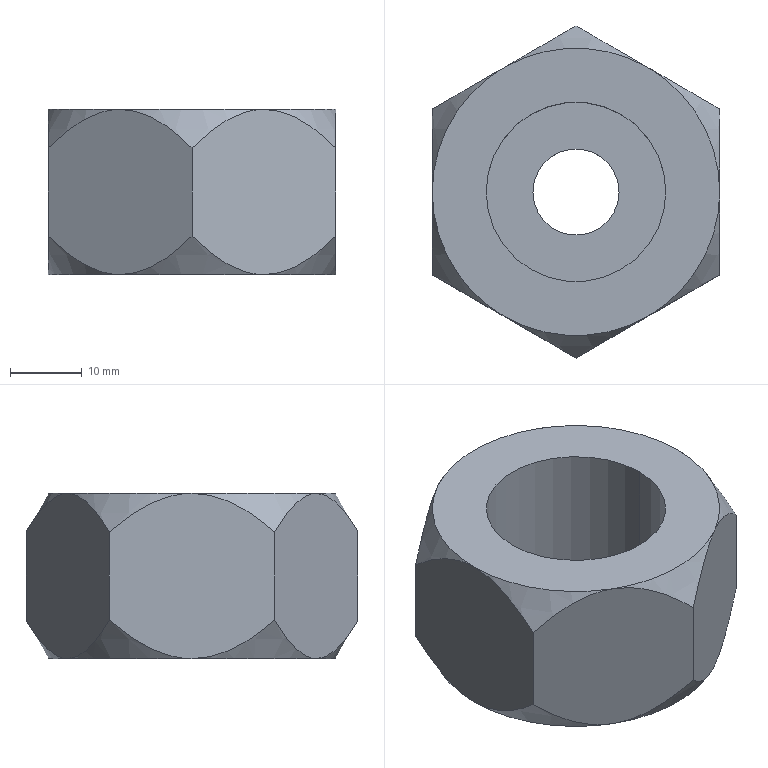Part | SolidWorks | features ICE 3, Extrusion 1, MirrorPattern 1 | 1 solid | 25 faces | box 40 x 46.188 x 23 mm | volume 22052 mm3 | cone 12 | plane 9 | cylinder 4 | commonest cylinder face diameters 12 x2 25 x2
STEP:
#1=CARTESIAN_POINT('',(-6.,0.,-11.5));
#2=VERTEX_POINT('',#1);
#3=CARTESIAN_POINT('',(6.,0.,-11.5));
#4=VERTEX_POINT('',#3);
#5=CARTESIAN_POINT('',(0.,0.,-11.5));
#6=DIRECTION('',(0.,0.,1.));
#7=DIRECTION('',(1.,0.,0.));
#8=AXIS2_PLACEMENT_3D('',#5,#6,#7);
#9=CIRCLE('',#8,6.);
#10=EDGE_CURVE('',#2,#4,#9,.T.);
#11=ORIENTED_EDGE('',*,*,#10,.F.);
#12=CARTESIAN_POINT('',(-6.,0.,-6.5));
#13=VERTEX_POINT('',#12);
#14=CARTESIAN_POINT('',(-6.,0.,-24.5));
#15=DIRECTION('',(0.,0.,1.));
#16=VECTOR('',#15,1000.);
#17=LINE('',#14,#16);
#18=EDGE_CURVE('',#2,#13,#17,.T.);
#19=ORIENTED_EDGE('',*,*,#18,.T.);
#20=CARTESIAN_POINT('',(6.,0.,-6.5));
#21=VERTEX_POINT('',#20);
#22=CARTESIAN_POINT('',(0.,0.,-6.5));
#23=DIRECTION('',(0.,0.,1.));
#24=DIRECTION('',(1.,0.,0.));
#25=AXIS2_PLACEMENT_3D('',#22,#23,#24);
#26=CIRCLE('',#25,6.);
#27=EDGE_CURVE('',#13,#21,#26,.T.);
#28=ORIENTED_EDGE('',*,*,#27,.T.);
#29=CARTESIAN_POINT('',(6.,0.,-24.5));
#30=DIRECTION('',(0.,0.,1.));
#31=VECTOR('',#30,1000.);
#32=LINE('',#29,#31);
#33=EDGE_CURVE('',#4,#21,#32,.T.);
#34=ORIENTED_EDGE('',*,*,#33,.F.);
#35=EDGE_LOOP('',(#11,#19,#28,#34));
#36=FACE_OUTER_BOUND('',#35,.T.);
#37=CARTESIAN_POINT('',(0.,0.,-24.5));
#38=DIRECTION('',(0.,0.,1.));
#39=DIRECTION('',(1.,0.,0.));
#40=AXIS2_PLACEMENT_3D('',#37,#38,#39);
#41=CYLINDRICAL_SURFACE('',#40,6.);
#42=ADVANCED_FACE('',(#36),#41,.F.);
#43=CARTESIAN_POINT('',(-12.5,0.,-6.5));
#44=VERTEX_POINT('',#43);
#45=CARTESIAN_POINT('',(12.5,0.,-6.5));
#46=VERTEX_POINT('',#45);
#47=CARTESIAN_POINT('',(0.,0.,-6.5));
#48=DIRECTION('',(0.,0.,1.));
#49=DIRECTION('',(1.,0.,0.));
#50=AXIS2_PLACEMENT_3D('',#47,#48,#49);
#51=CIRCLE('',#50,12.5);
#52=EDGE_CURVE('',#44,#46,#51,.T.);
#53=ORIENTED_EDGE('',*,*,#52,.F.);
#54=CARTESIAN_POINT('',(-12.5,0.,11.5));
#55=VERTEX_POINT('',#54);
#56=CARTESIAN_POINT('',(-12.5,0.,-6.5));
#57=DIRECTION('',(0.,0.,1.));
#58=VECTOR('',#57,1000.);
#59=LINE('',#56,#58);
#60=EDGE_CURVE('',#44,#55,#59,.T.);
#61=ORIENTED_EDGE('',*,*,#60,.T.);
#62=CARTESIAN_POINT('',(12.5,0.,11.5));
#63=VERTEX_POINT('',#62);
#64=CARTESIAN_POINT('',(0.,0.,11.5));
#65=DIRECTION('',(0.,0.,1.));
#66=DIRECTION('',(1.,0.,0.));
#67=AXIS2_PLACEMENT_3D('',#64,#65,#66);
#68=CIRCLE('',#67,12.5);
#69=EDGE_CURVE('',#55,#63,#68,.T.);
#70=ORIENTED_EDGE('',*,*,#69,.T.);
#71=CARTESIAN_POINT('',(12.5,0.,-6.5));
#72=DIRECTION('',(0.,0.,1.));
#73=VECTOR('',#72,1000.);
#74=LINE('',#71,#73);
#75=EDGE_CURVE('',#46,#63,#74,.T.);
#76=ORIENTED_EDGE('',*,*,#75,.F.);
#77=EDGE_LOOP('',(#53,#61,#70,#76));
#78=FACE_OUTER_BOUND('',#77,.T.);
#79=CARTESIAN_POINT('',(0.,0.,-6.5));
#80=DIRECTION('',(0.,0.,1.));
#81=DIRECTION('',(1.,0.,0.));
#82=AXIS2_PLACEMENT_3D('',#79,#80,#81);
#83=CYLINDRICAL_SURFACE('',#82,12.5);
#84=ADVANCED_FACE('',(#78),#83,.F.);
#85=CARTESIAN_POINT('',(20.,11.547,6.141));
#86=VERTEX_POINT('',#85);
#87=CARTESIAN_POINT('',(20.,11.547,-6.141));
#88=VERTEX_POINT('',#87);
#89=CARTESIAN_POINT('',(20.,11.547,11.5));
#90=DIRECTION('',(0.,0.,-1.));
#91=VECTOR('',#90,1000.);
#92=LINE('',#89,#91);
#93=EDGE_CURVE('',#86,#88,#92,.T.);
#94=ORIENTED_EDGE('',*,*,#93,.T.);
#95=CARTESIAN_POINT('',(10.,17.321,-11.5));
#96=VERTEX_POINT('',#95);
#97=CARTESIAN_POINT('',(20.,11.547,-6.141));
#98=CARTESIAN_POINT('',(19.289,11.958,-6.852));
#99=CARTESIAN_POINT('',(18.557,12.38,-7.528));
#100=CARTESIAN_POINT('',(17.035,13.259,-8.777));
#101=CARTESIAN_POINT('',(16.246,13.715,-9.351));
#102=CARTESIAN_POINT('',(14.996,14.436,-10.097));
#103=CARTESIAN_POINT('',(14.566,14.684,-10.327));
#104=CARTESIAN_POINT('',(13.688,15.191,-10.734));
#105=CARTESIAN_POINT('',(13.243,15.448,-10.909));
#106=CARTESIAN_POINT('',(12.34,15.97,-11.197));
#107=CARTESIAN_POINT('',(11.881,16.235,-11.309));
#108=CARTESIAN_POINT('',(10.947,16.774,-11.461));
#109=CARTESIAN_POINT('',(10.47,17.049,-11.5));
#110=CARTESIAN_POINT('',(10.,17.321,-11.5));
#111=B_SPLINE_CURVE_WITH_KNOTS('',3,(#97,#98,#99,#100,#101,#102,#103,#104,#105,#106,#107,#108,#109,#110),.UNSPECIFIED.,.F.,.F.,(4,2,2,2,2,2,4),(0.000000303,0.003232,0.006463,0.008079,0.009695,0.01131,0.01293),.UNSPECIFIED.);
#112=EDGE_CURVE('',#88,#96,#111,.T.);
#113=ORIENTED_EDGE('',*,*,#112,.T.);
#114=CARTESIAN_POINT('',(0.,23.094,-6.141));
#115=VERTEX_POINT('',#114);
#116=CARTESIAN_POINT('',(10.,17.321,-11.5));
#117=CARTESIAN_POINT('',(9.062,17.862,-11.5));
#118=CARTESIAN_POINT('',(8.137,18.396,-11.347));
#119=CARTESIAN_POINT('',(6.768,19.187,-10.913));
#120=CARTESIAN_POINT('',(6.321,19.444,-10.737));
#121=CARTESIAN_POINT('',(5.452,19.946,-10.336));
#122=CARTESIAN_POINT('',(5.028,20.191,-10.11));
#123=CARTESIAN_POINT('',(4.197,20.671,-9.616));
#124=CARTESIAN_POINT('',(3.791,20.905,-9.349));
#125=CARTESIAN_POINT('',(2.992,21.367,-8.779));
#126=CARTESIAN_POINT('',(2.599,21.594,-8.476));
#127=CARTESIAN_POINT('',(1.447,22.258,-7.532));
#128=CARTESIAN_POINT('',(0.7124,22.683,-6.853));
#129=CARTESIAN_POINT('',(0.,23.094,-6.141));
#130=B_SPLINE_CURVE_WITH_KNOTS('',3,(#116,#117,#118,#119,#120,#121,#122,#123,#124,#125,#126,#127,#128,#129),.UNSPECIFIED.,.F.,.F.,(4,2,2,2,2,2,4),(0.01293,0.01615,0.01777,0.01938,0.02099,0.02261,0.02583),.UNSPECIFIED.);
#131=EDGE_CURVE('',#96,#115,#130,.T.);
#132=ORIENTED_EDGE('',*,*,#131,.T.);
#133=CARTESIAN_POINT('',(0.,23.094,6.141));
#134=VERTEX_POINT('',#133);
#135=CARTESIAN_POINT('',(0.,23.094,11.5));
#136=DIRECTION('',(0.,0.,-1.));
#137=VECTOR('',#136,1000.);
#138=LINE('',#135,#137);
#139=EDGE_CURVE('',#134,#115,#138,.T.);
#140=ORIENTED_EDGE('',*,*,#139,.F.);
#141=CARTESIAN_POINT('',(10.,17.321,11.5));
#142=VERTEX_POINT('',#141);
#143=CARTESIAN_POINT('',(10.,17.321,11.5));
#144=CARTESIAN_POINT('',(9.062,17.862,11.5));
#145=CARTESIAN_POINT('',(8.137,18.396,11.347));
#146=CARTESIAN_POINT('',(6.768,19.187,10.913));
#147=CARTESIAN_POINT('',(6.321,19.444,10.737));
#148=CARTESIAN_POINT('',(5.452,19.946,10.336));
#149=CARTESIAN_POINT('',(5.028,20.191,10.11));
#150=CARTESIAN_POINT('',(4.197,20.671,9.616));
#151=CARTESIAN_POINT('',(3.791,20.905,9.349));
#152=CARTESIAN_POINT('',(2.992,21.367,8.779));
#153=CARTESIAN_POINT('',(2.599,21.594,8.476));
#154=CARTESIAN_POINT('',(1.447,22.258,7.532));
#155=CARTESIAN_POINT('',(0.7124,22.683,6.853));
#156=CARTESIAN_POINT('',(0.,23.094,6.141));
#157=B_SPLINE_CURVE_WITH_KNOTS('',3,(#143,#144,#145,#146,#147,#148,#149,#150,#151,#152,#153,#154,#155,#156),.UNSPECIFIED.,.F.,.F.,(4,2,2,2,2,2,4),(0.01293,0.01615,0.01777,0.01938,0.02099,0.02261,0.02583),.UNSPECIFIED.);
#158=EDGE_CURVE('',#142,#134,#157,.T.);
#159=ORIENTED_EDGE('',*,*,#158,.F.);
#160=CARTESIAN_POINT('',(20.,11.547,6.141));
#161=CARTESIAN_POINT('',(19.289,11.958,6.852));
#162=CARTESIAN_POINT('',(18.557,12.38,7.528));
#163=CARTESIAN_POINT('',(17.035,13.259,8.777));
#164=CARTESIAN_POINT('',(16.246,13.715,9.351));
#165=CARTESIAN_POINT('',(14.996,14.436,10.097));
#166=CARTESIAN_POINT('',(14.566,14.684,10.327));
#167=CARTESIAN_POINT('',(13.688,15.191,10.734));
#168=CARTESIAN_POINT('',(13.243,15.448,10.909));
#169=CARTESIAN_POINT('',(12.34,15.97,11.197));
#170=CARTESIAN_POINT('',(11.881,16.235,11.309));
#171=CARTESIAN_POINT('',(10.947,16.774,11.461));
#172=CARTESIAN_POINT('',(10.47,17.049,11.5));
#173=CARTESIAN_POINT('',(10.,17.321,11.5));
#174=B_SPLINE_CURVE_WITH_KNOTS('',3,(#160,#161,#162,#163,#164,#165,#166,#167,#168,#169,#170,#171,#172,#173),.UNSPECIFIED.,.F.,.F.,(4,2,2,2,2,2,4),(0.000000303,0.003232,0.006463,0.008079,0.009695,0.01131,0.01293),.UNSPECIFIED.);
#175=EDGE_CURVE('',#86,#142,#174,.T.);
#176=ORIENTED_EDGE('',*,*,#175,.F.);
#177=EDGE_LOOP('',(#94,#113,#132,#140,#159,#176));
#178=FACE_OUTER_BOUND('',#177,.T.);
#179=CARTESIAN_POINT('',(20.,11.547,11.5));
#180=DIRECTION('',(-0.5,-0.866,0.));
#181=DIRECTION('',(0.866,-0.5,0.));
#182=AXIS2_PLACEMENT_3D('',#179,#180,#181);
#183=PLANE('',#182);
#184=ADVANCED_FACE('',(#178),#183,.F.);
#185=ORIENTED_EDGE('',*,*,#139,.T.);
#186=CARTESIAN_POINT('',(-10.,17.321,-11.5));
#187=VERTEX_POINT('',#186);
#188=CARTESIAN_POINT('',(0.,23.094,-6.141));
#189=CARTESIAN_POINT('',(-0.7114,22.683,-6.852));
#190=CARTESIAN_POINT('',(-1.443,22.261,-7.528));
#191=CARTESIAN_POINT('',(-2.965,21.382,-8.777));
#192=CARTESIAN_POINT('',(-3.754,20.926,-9.351));
#193=CARTESIAN_POINT('',(-5.004,20.205,-10.097));
#194=CARTESIAN_POINT('',(-5.434,19.957,-10.327));
#195=CARTESIAN_POINT('',(-6.312,19.45,-10.734));
#196=CARTESIAN_POINT('',(-6.757,19.193,-10.909));
#197=CARTESIAN_POINT('',(-7.66,18.671,-11.197));
#198=CARTESIAN_POINT('',(-8.119,18.406,-11.309));
#199=CARTESIAN_POINT('',(-9.053,17.867,-11.461));
#200=CARTESIAN_POINT('',(-9.53,17.592,-11.5));
#201=CARTESIAN_POINT('',(-10.,17.321,-11.5));
#202=B_SPLINE_CURVE_WITH_KNOTS('',3,(#188,#189,#190,#191,#192,#193,#194,#195,#196,#197,#198,#199,#200,#201),.UNSPECIFIED.,.F.,.F.,(4,2,2,2,2,2,4),(0.000000303,0.003232,0.006463,0.008079,0.009695,0.01131,0.01293),.UNSPECIFIED.);
#203=EDGE_CURVE('',#115,#187,#202,.T.);
#204=ORIENTED_EDGE('',*,*,#203,.T.);
#205=CARTESIAN_POINT('',(-20.,11.547,-6.141));
#206=VERTEX_POINT('',#205);
#207=CARTESIAN_POINT('',(-10.,17.321,-11.5));
#208=CARTESIAN_POINT('',(-10.938,16.779,-11.5));
#209=CARTESIAN_POINT('',(-11.863,16.245,-11.347));
#210=CARTESIAN_POINT('',(-13.232,15.454,-10.913));
#211=CARTESIAN_POINT('',(-13.679,15.197,-10.737));
#212=CARTESIAN_POINT('',(-14.548,14.695,-10.336));
#213=CARTESIAN_POINT('',(-14.972,14.45,-10.11));
#214=CARTESIAN_POINT('',(-15.803,13.97,-9.616));
#215=CARTESIAN_POINT('',(-16.209,13.736,-9.349));
#216=CARTESIAN_POINT('',(-17.008,13.274,-8.779));
#217=CARTESIAN_POINT('',(-17.401,13.047,-8.476));
#218=CARTESIAN_POINT('',(-18.553,12.383,-7.532));
#219=CARTESIAN_POINT('',(-19.288,11.958,-6.853));
#220=CARTESIAN_POINT('',(-20.,11.547,-6.141));
#221=B_SPLINE_CURVE_WITH_KNOTS('',3,(#207,#208,#209,#210,#211,#212,#213,#214,#215,#216,#217,#218,#219,#220),.UNSPECIFIED.,.F.,.F.,(4,2,2,2,2,2,4),(0.01293,0.01615,0.01777,0.01938,0.02099,0.02261,0.02583),.UNSPECIFIED.);
#222=EDGE_CURVE('',#187,#206,#221,.T.);
#223=ORIENTED_EDGE('',*,*,#222,.T.);
#224=CARTESIAN_POINT('',(-20.,11.547,6.141));
#225=VERTEX_POINT('',#224);
#226=CARTESIAN_POINT('',(-20.,11.547,11.5));
#227=DIRECTION('',(0.,0.,-1.));
#228=VECTOR('',#227,1000.);
#229=LINE('',#226,#228);
#230=EDGE_CURVE('',#225,#206,#229,.T.);
#231=ORIENTED_EDGE('',*,*,#230,.F.);
#232=CARTESIAN_POINT('',(-10.,17.321,11.5));
#233=VERTEX_POINT('',#232);
#234=CARTESIAN_POINT('',(-10.,17.321,11.5));
#235=CARTESIAN_POINT('',(-10.938,16.779,11.5));
#236=CARTESIAN_POINT('',(-11.863,16.245,11.347));
#237=CARTESIAN_POINT('',(-13.232,15.454,10.913));
#238=CARTESIAN_POINT('',(-13.679,15.197,10.737));
#239=CARTESIAN_POINT('',(-14.548,14.695,10.336));
#240=CARTESIAN_POINT('',(-14.972,14.45,10.11));
#241=CARTESIAN_POINT('',(-15.803,13.97,9.616));
#242=CARTESIAN_POINT('',(-16.209,13.736,9.349));
#243=CARTESIAN_POINT('',(-17.008,13.274,8.779));
#244=CARTESIAN_POINT('',(-17.401,13.047,8.476));
#245=CARTESIAN_POINT('',(-18.553,12.383,7.532));
#246=CARTESIAN_POINT('',(-19.288,11.958,6.853));
#247=CARTESIAN_POINT('',(-20.,11.547,6.141));
#248=B_SPLINE_CURVE_WITH_KNOTS('',3,(#234,#235,#236,#237,#238,#239,#240,#241,#242,#243,#244,#245,#246,#247),.UNSPECIFIED.,.F.,.F.,(4,2,2,2,2,2,4),(0.01293,0.01615,0.01777,0.01938,0.02099,0.02261,0.02583),.UNSPECIFIED.);
#249=EDGE_CURVE('',#233,#225,#248,.T.);
#250=ORIENTED_EDGE('',*,*,#249,.F.);
#251=CARTESIAN_POINT('',(0.,23.094,6.141));
#252=CARTESIAN_POINT('',(-0.7114,22.683,6.852));
#253=CARTESIAN_POINT('',(-1.443,22.261,7.528));
#254=CARTESIAN_POINT('',(-2.965,21.382,8.777));
#255=CARTESIAN_POINT('',(-3.754,20.926,9.351));
#256=CARTESIAN_POINT('',(-5.004,20.205,10.097));
#257=CARTESIAN_POINT('',(-5.434,19.957,10.327));
#258=CARTESIAN_POINT('',(-6.312,19.45,10.734));
#259=CARTESIAN_POINT('',(-6.757,19.193,10.909));
#260=CARTESIAN_POINT('',(-7.66,18.671,11.197));
#261=CARTESIAN_POINT('',(-8.119,18.406,11.309));
#262=CARTESIAN_POINT('',(-9.053,17.867,11.461));
#263=CARTESIAN_POINT('',(-9.53,17.592,11.5));
#264=CARTESIAN_POINT('',(-10.,17.321,11.5));
#265=B_SPLINE_CURVE_WITH_KNOTS('',3,(#251,#252,#253,#254,#255,#256,#257,#258,#259,#260,#261,#262,#263,#264),.UNSPECIFIED.,.F.,.F.,(4,2,2,2,2,2,4),(0.000000303,0.003232,0.006463,0.008079,0.009695,0.01131,0.01293),.UNSPECIFIED.);
#266=EDGE_CURVE('',#134,#233,#265,.T.);
#267=ORIENTED_EDGE('',*,*,#266,.F.);
#268=EDGE_LOOP('',(#185,#204,#223,#231,#250,#267));
#269=FACE_OUTER_BOUND('',#268,.T.);
#270=CARTESIAN_POINT('',(0.,23.094,11.5));
#271=DIRECTION('',(0.5,-0.866,0.));
#272=DIRECTION('',(0.866,0.5,0.));
#273=AXIS2_PLACEMENT_3D('',#270,#271,#272);
#274=PLANE('',#273);
#275=ADVANCED_FACE('',(#269),#274,.F.);
#276=ORIENTED_EDGE('',*,*,#230,.T.);
#277=CARTESIAN_POINT('',(-20.,0.,-11.5));
#278=VERTEX_POINT('',#277);
#279=CARTESIAN_POINT('',(-20.,11.547,-6.141));
#280=CARTESIAN_POINT('',(-20.,11.14,-6.493));
#281=CARTESIAN_POINT('',(-20.,10.726,-6.838));
#282=CARTESIAN_POINT('',(-20.,9.877,-7.511));
#283=CARTESIAN_POINT('',(-20.,9.442,-7.84));
#284=CARTESIAN_POINT('',(-20.,8.115,-8.783));
#285=CARTESIAN_POINT('',(-20.,7.2,-9.358));
#286=CARTESIAN_POINT('',(-20.,5.76,-10.101));
#287=CARTESIAN_POINT('',(-20.,5.269,-10.328));
#288=CARTESIAN_POINT('',(-20.,4.26,-10.733));
#289=CARTESIAN_POINT('',(-20.,3.74,-10.911));
#290=CARTESIAN_POINT('',(-20.,2.693,-11.199));
#291=CARTESIAN_POINT('',(-20.,2.164,-11.31));
#292=CARTESIAN_POINT('',(-20.,1.092,-11.461));
#293=CARTESIAN_POINT('',(-20.,0.5475,-11.5));
#294=CARTESIAN_POINT('',(-20.,0.,-11.5));
#295=B_SPLINE_CURVE_WITH_KNOTS('',3,(#279,#280,#281,#282,#283,#284,#285,#286,#287,#288,#289,#290,#291,#292,#293,#294),.UNSPECIFIED.,.F.,.F.,(4,2,2,2,2,2,2,4),(0.02147,0.02307,0.02467,0.02788,0.02948,0.03108,0.03268,0.03428),.UNSPECIFIED.);
#296=EDGE_CURVE('',#206,#278,#295,.T.);
#297=ORIENTED_EDGE('',*,*,#296,.T.);
#298=CARTESIAN_POINT('',(-20.,-11.547,-6.141));
#299=VERTEX_POINT('',#298);
#300=CARTESIAN_POINT('',(-20.,0.,-11.5));
#301=CARTESIAN_POINT('',(-20.,-1.096,-11.5));
#302=CARTESIAN_POINT('',(-20.,-2.166,-11.344));
#303=CARTESIAN_POINT('',(-20.,-3.74,-10.911));
#304=CARTESIAN_POINT('',(-20.,-4.26,-10.733));
#305=CARTESIAN_POINT('',(-20.,-5.268,-10.328));
#306=CARTESIAN_POINT('',(-20.,-5.759,-10.101));
#307=CARTESIAN_POINT('',(-20.,-7.198,-9.359));
#308=CARTESIAN_POINT('',(-20.,-8.114,-8.784));
#309=CARTESIAN_POINT('',(-20.,-9.443,-7.839));
#310=CARTESIAN_POINT('',(-20.,-9.878,-7.511));
#311=CARTESIAN_POINT('',(-20.,-10.726,-6.838));
#312=CARTESIAN_POINT('',(-20.,-11.14,-6.493));
#313=CARTESIAN_POINT('',(-20.,-11.547,-6.141));
#314=B_SPLINE_CURVE_WITH_KNOTS('',3,(#300,#301,#302,#303,#304,#305,#306,#307,#308,#309,#310,#311,#312,#313),.UNSPECIFIED.,.F.,.F.,(4,2,2,2,2,2,4),(0.03428,0.03749,0.03909,0.04069,0.04389,0.0455,0.0471),.UNSPECIFIED.);
#315=EDGE_CURVE('',#278,#299,#314,.T.);
#316=ORIENTED_EDGE('',*,*,#315,.T.);
#317=CARTESIAN_POINT('',(-20.,-11.547,6.141));
#318=VERTEX_POINT('',#317);
#319=CARTESIAN_POINT('',(-20.,-11.547,11.5));
#320=DIRECTION('',(0.,0.,-1.));
#321=VECTOR('',#320,1000.);
#322=LINE('',#319,#321);
#323=EDGE_CURVE('',#318,#299,#322,.T.);
#324=ORIENTED_EDGE('',*,*,#323,.F.);
#325=CARTESIAN_POINT('',(-20.,0.,11.5));
#326=VERTEX_POINT('',#325);
#327=CARTESIAN_POINT('',(-20.,0.,11.5));
#328=CARTESIAN_POINT('',(-20.,-1.096,11.5));
#329=CARTESIAN_POINT('',(-20.,-2.166,11.344));
#330=CARTESIAN_POINT('',(-20.,-3.74,10.911));
#331=CARTESIAN_POINT('',(-20.,-4.26,10.733));
#332=CARTESIAN_POINT('',(-20.,-5.268,10.328));
#333=CARTESIAN_POINT('',(-20.,-5.759,10.101));
#334=CARTESIAN_POINT('',(-20.,-7.198,9.359));
#335=CARTESIAN_POINT('',(-20.,-8.114,8.784));
#336=CARTESIAN_POINT('',(-20.,-9.443,7.839));
#337=CARTESIAN_POINT('',(-20.,-9.878,7.511));
#338=CARTESIAN_POINT('',(-20.,-10.726,6.838));
#339=CARTESIAN_POINT('',(-20.,-11.14,6.493));
#340=CARTESIAN_POINT('',(-20.,-11.547,6.141));
#341=B_SPLINE_CURVE_WITH_KNOTS('',3,(#327,#328,#329,#330,#331,#332,#333,#334,#335,#336,#337,#338,#339,#340),.UNSPECIFIED.,.F.,.F.,(4,2,2,2,2,2,4),(0.03428,0.03749,0.03909,0.04069,0.04389,0.0455,0.0471),.UNSPECIFIED.);
#342=EDGE_CURVE('',#326,#318,#341,.T.);
#343=ORIENTED_EDGE('',*,*,#342,.F.);
#344=CARTESIAN_POINT('',(-20.,11.547,6.141));
#345=CARTESIAN_POINT('',(-20.,11.14,6.493));
#346=CARTESIAN_POINT('',(-20.,10.726,6.838));
#347=CARTESIAN_POINT('',(-20.,9.877,7.511));
#348=CARTESIAN_POINT('',(-20.,9.442,7.84));
#349=CARTESIAN_POINT('',(-20.,8.115,8.783));
#350=CARTESIAN_POINT('',(-20.,7.2,9.358));
#351=CARTESIAN_POINT('',(-20.,5.76,10.101));
#352=CARTESIAN_POINT('',(-20.,5.269,10.328));
#353=CARTESIAN_POINT('',(-20.,4.26,10.733));
#354=CARTESIAN_POINT('',(-20.,3.74,10.911));
#355=CARTESIAN_POINT('',(-20.,2.693,11.199));
#356=CARTESIAN_POINT('',(-20.,2.164,11.31));
#357=CARTESIAN_POINT('',(-20.,1.092,11.461));
#358=CARTESIAN_POINT('',(-20.,0.5475,11.5));
#359=CARTESIAN_POINT('',(-20.,0.,11.5));
#360=B_SPLINE_CURVE_WITH_KNOTS('',3,(#344,#345,#346,#347,#348,#349,#350,#351,#352,#353,#354,#355,#356,#357,#358,#359),.UNSPECIFIED.,.F.,.F.,(4,2,2,2,2,2,2,4),(0.02147,0.02307,0.02467,0.02788,0.02948,0.03108,0.03268,0.03428),.UNSPECIFIED.);
#361=EDGE_CURVE('',#225,#326,#360,.T.);
#362=ORIENTED_EDGE('',*,*,#361,.F.);
#363=EDGE_LOOP('',(#276,#297,#316,#324,#343,#362));
#364=FACE_OUTER_BOUND('',#363,.T.);
#365=CARTESIAN_POINT('',(-20.,11.547,11.5));
#366=DIRECTION('',(1.,0.,0.));
#367=DIRECTION('',(0.,1.,0.));
#368=AXIS2_PLACEMENT_3D('',#365,#366,#367);
#369=PLANE('',#368);
#370=ADVANCED_FACE('',(#364),#369,.F.);
#371=ORIENTED_EDGE('',*,*,#323,.T.);
#372=CARTESIAN_POINT('',(-10.,-17.321,-11.5));
#373=VERTEX_POINT('',#372);
#374=CARTESIAN_POINT('',(-20.,-11.547,-6.141));
#375=CARTESIAN_POINT('',(-19.289,-11.958,-6.852));
#376=CARTESIAN_POINT('',(-18.557,-12.38,-7.528));
#377=CARTESIAN_POINT('',(-17.035,-13.259,-8.777));
#378=CARTESIAN_POINT('',(-16.246,-13.715,-9.351));
#379=CARTESIAN_POINT('',(-14.996,-14.436,-10.097));
#380=CARTESIAN_POINT('',(-14.566,-14.684,-10.327));
#381=CARTESIAN_POINT('',(-13.688,-15.191,-10.734));
#382=CARTESIAN_POINT('',(-13.243,-15.448,-10.909));
#383=CARTESIAN_POINT('',(-12.34,-15.97,-11.197));
#384=CARTESIAN_POINT('',(-11.881,-16.235,-11.309));
#385=CARTESIAN_POINT('',(-10.947,-16.774,-11.461));
#386=CARTESIAN_POINT('',(-10.47,-17.049,-11.5));
#387=CARTESIAN_POINT('',(-10.,-17.321,-11.5));
#388=B_SPLINE_CURVE_WITH_KNOTS('',3,(#374,#375,#376,#377,#378,#379,#380,#381,#382,#383,#384,#385,#386,#387),.UNSPECIFIED.,.F.,.F.,(4,2,2,2,2,2,4),(0.000000303,0.003232,0.006463,0.008079,0.009695,0.01131,0.01293),.UNSPECIFIED.);
#389=EDGE_CURVE('',#299,#373,#388,.T.);
#390=ORIENTED_EDGE('',*,*,#389,.T.);
#391=CARTESIAN_POINT('',(0.,-23.094,-6.141));
#392=VERTEX_POINT('',#391);
#393=CARTESIAN_POINT('',(-10.,-17.321,-11.5));
#394=CARTESIAN_POINT('',(-9.062,-17.862,-11.5));
#395=CARTESIAN_POINT('',(-8.137,-18.396,-11.347));
#396=CARTESIAN_POINT('',(-6.768,-19.187,-10.913));
#397=CARTESIAN_POINT('',(-6.321,-19.444,-10.737));
#398=CARTESIAN_POINT('',(-5.452,-19.946,-10.336));
#399=CARTESIAN_POINT('',(-5.028,-20.191,-10.11));
#400=CARTESIAN_POINT('',(-4.197,-20.671,-9.616));
#401=CARTESIAN_POINT('',(-3.791,-20.905,-9.349));
#402=CARTESIAN_POINT('',(-2.992,-21.367,-8.779));
#403=CARTESIAN_POINT('',(-2.599,-21.594,-8.476));
#404=CARTESIAN_POINT('',(-1.447,-22.258,-7.532));
#405=CARTESIAN_POINT('',(-0.7124,-22.683,-6.853));
#406=CARTESIAN_POINT('',(0.,-23.094,-6.141));
#407=B_SPLINE_CURVE_WITH_KNOTS('',3,(#393,#394,#395,#396,#397,#398,#399,#400,#401,#402,#403,#404,#405,#406),.UNSPECIFIED.,.F.,.F.,(4,2,2,2,2,2,4),(0.01293,0.01615,0.01777,0.01938,0.02099,0.02261,0.02583),.UNSPECIFIED.);
#408=EDGE_CURVE('',#373,#392,#407,.T.);
#409=ORIENTED_EDGE('',*,*,#408,.T.);
#410=CARTESIAN_POINT('',(0.,-23.094,6.141));
#411=VERTEX_POINT('',#410);
#412=CARTESIAN_POINT('',(0.,-23.094,11.5));
#413=DIRECTION('',(0.,0.,-1.));
#414=VECTOR('',#413,1000.);
#415=LINE('',#412,#414);
#416=EDGE_CURVE('',#411,#392,#415,.T.);
#417=ORIENTED_EDGE('',*,*,#416,.F.);
#418=CARTESIAN_POINT('',(-10.,-17.321,11.5));
#419=VERTEX_POINT('',#418);
#420=CARTESIAN_POINT('',(-10.,-17.321,11.5));
#421=CARTESIAN_POINT('',(-9.062,-17.862,11.5));
#422=CARTESIAN_POINT('',(-8.137,-18.396,11.347));
#423=CARTESIAN_POINT('',(-6.768,-19.187,10.913));
#424=CARTESIAN_POINT('',(-6.321,-19.444,10.737));
#425=CARTESIAN_POINT('',(-5.452,-19.946,10.336));
#426=CARTESIAN_POINT('',(-5.028,-20.191,10.11));
#427=CARTESIAN_POINT('',(-4.197,-20.671,9.616));
#428=CARTESIAN_POINT('',(-3.791,-20.905,9.349));
#429=CARTESIAN_POINT('',(-2.992,-21.367,8.779));
#430=CARTESIAN_POINT('',(-2.599,-21.594,8.476));
#431=CARTESIAN_POINT('',(-1.447,-22.258,7.532));
#432=CARTESIAN_POINT('',(-0.7124,-22.683,6.853));
#433=CARTESIAN_POINT('',(0.,-23.094,6.141));
#434=B_SPLINE_CURVE_WITH_KNOTS('',3,(#420,#421,#422,#423,#424,#425,#426,#427,#428,#429,#430,#431,#432,#433),.UNSPECIFIED.,.F.,.F.,(4,2,2,2,2,2,4),(0.01293,0.01615,0.01777,0.01938,0.02099,0.02261,0.02583),.UNSPECIFIED.);
#435=EDGE_CURVE('',#419,#411,#434,.T.);
#436=ORIENTED_EDGE('',*,*,#435,.F.);
#437=CARTESIAN_POINT('',(-20.,-11.547,6.141));
#438=CARTESIAN_POINT('',(-19.289,-11.958,6.852));
#439=CARTESIAN_POINT('',(-18.557,-12.38,7.528));
#440=CARTESIAN_POINT('',(-17.035,-13.259,8.777));
#441=CARTESIAN_POINT('',(-16.246,-13.715,9.351));
#442=CARTESIAN_POINT('',(-14.996,-14.436,10.097));
#443=CARTESIAN_POINT('',(-14.566,-14.684,10.327));
#444=CARTESIAN_POINT('',(-13.688,-15.191,10.734));
#445=CARTESIAN_POINT('',(-13.243,-15.448,10.909));
#446=CARTESIAN_POINT('',(-12.34,-15.97,11.197));
#447=CARTESIAN_POINT('',(-11.881,-16.235,11.309));
#448=CARTESIAN_POINT('',(-10.947,-16.774,11.461));
#449=CARTESIAN_POINT('',(-10.47,-17.049,11.5));
#450=CARTESIAN_POINT('',(-10.,-17.321,11.5));
#451=B_SPLINE_CURVE_WITH_KNOTS('',3,(#437,#438,#439,#440,#441,#442,#443,#444,#445,#446,#447,#448,#449,#450),.UNSPECIFIED.,.F.,.F.,(4,2,2,2,2,2,4),(0.000000303,0.003232,0.006463,0.008079,0.009695,0.01131,0.01293),.UNSPECIFIED.);
#452=EDGE_CURVE('',#318,#419,#451,.T.);
#453=ORIENTED_EDGE('',*,*,#452,.F.);
#454=EDGE_LOOP('',(#371,#390,#409,#417,#436,#453));
#455=FACE_OUTER_BOUND('',#454,.T.);
#456=CARTESIAN_POINT('',(-20.,-11.547,11.5));
#457=DIRECTION('',(0.5,0.866,0.));
#458=DIRECTION('',(-0.866,0.5,0.));
#459=AXIS2_PLACEMENT_3D('',#456,#457,#458);
#460=PLANE('',#459);
#461=ADVANCED_FACE('',(#455),#460,.F.);
#462=ORIENTED_EDGE('',*,*,#416,.T.);
#463=CARTESIAN_POINT('',(10.,-17.321,-11.5));
#464=VERTEX_POINT('',#463);
#465=CARTESIAN_POINT('',(0.,-23.094,-6.141));
#466=CARTESIAN_POINT('',(0.7114,-22.683,-6.852));
#467=CARTESIAN_POINT('',(1.443,-22.261,-7.528));
#468=CARTESIAN_POINT('',(2.965,-21.382,-8.777));
#469=CARTESIAN_POINT('',(3.754,-20.926,-9.351));
#470=CARTESIAN_POINT('',(5.004,-20.205,-10.097));
#471=CARTESIAN_POINT('',(5.434,-19.957,-10.327));
#472=CARTESIAN_POINT('',(6.312,-19.45,-10.734));
#473=CARTESIAN_POINT('',(6.757,-19.193,-10.909));
#474=CARTESIAN_POINT('',(7.66,-18.671,-11.197));
#475=CARTESIAN_POINT('',(8.119,-18.406,-11.309));
#476=CARTESIAN_POINT('',(9.053,-17.867,-11.461));
#477=CARTESIAN_POINT('',(9.53,-17.592,-11.5));
#478=CARTESIAN_POINT('',(10.,-17.321,-11.5));
#479=B_SPLINE_CURVE_WITH_KNOTS('',3,(#465,#466,#467,#468,#469,#470,#471,#472,#473,#474,#475,#476,#477,#478),.UNSPECIFIED.,.F.,.F.,(4,2,2,2,2,2,4),(0.000000303,0.003232,0.006463,0.008079,0.009695,0.01131,0.01293),.UNSPECIFIED.);
#480=EDGE_CURVE('',#392,#464,#479,.T.);
#481=ORIENTED_EDGE('',*,*,#480,.T.);
#482=CARTESIAN_POINT('',(20.,-11.547,-6.141));
#483=VERTEX_POINT('',#482);
#484=CARTESIAN_POINT('',(10.,-17.321,-11.5));
#485=CARTESIAN_POINT('',(10.938,-16.779,-11.5));
#486=CARTESIAN_POINT('',(11.863,-16.245,-11.347));
#487=CARTESIAN_POINT('',(13.232,-15.454,-10.913));
#488=CARTESIAN_POINT('',(13.679,-15.197,-10.737));
#489=CARTESIAN_POINT('',(14.548,-14.695,-10.336));
#490=CARTESIAN_POINT('',(14.972,-14.45,-10.11));
#491=CARTESIAN_POINT('',(15.803,-13.97,-9.616));
#492=CARTESIAN_POINT('',(16.209,-13.736,-9.349));
#493=CARTESIAN_POINT('',(17.008,-13.274,-8.779));
#494=CARTESIAN_POINT('',(17.401,-13.047,-8.476));
#495=CARTESIAN_POINT('',(18.553,-12.383,-7.532));
#496=CARTESIAN_POINT('',(19.288,-11.958,-6.853));
#497=CARTESIAN_POINT('',(20.,-11.547,-6.141));
#498=B_SPLINE_CURVE_WITH_KNOTS('',3,(#484,#485,#486,#487,#488,#489,#490,#491,#492,#493,#494,#495,#496,#497),.UNSPECIFIED.,.F.,.F.,(4,2,2,2,2,2,4),(0.01293,0.01615,0.01777,0.01938,0.02099,0.02261,0.02583),.UNSPECIFIED.);
#499=EDGE_CURVE('',#464,#483,#498,.T.);
#500=ORIENTED_EDGE('',*,*,#499,.T.);
#501=CARTESIAN_POINT('',(20.,-11.547,6.141));
#502=VERTEX_POINT('',#501);
#503=CARTESIAN_POINT('',(20.,-11.547,11.5));
#504=DIRECTION('',(0.,0.,-1.));
#505=VECTOR('',#504,1000.);
#506=LINE('',#503,#505);
#507=EDGE_CURVE('',#502,#483,#506,.T.);
#508=ORIENTED_EDGE('',*,*,#507,.F.);
#509=CARTESIAN_POINT('',(10.,-17.321,11.5));
#510=VERTEX_POINT('',#509);
#511=CARTESIAN_POINT('',(10.,-17.321,11.5));
#512=CARTESIAN_POINT('',(10.938,-16.779,11.5));
#513=CARTESIAN_POINT('',(11.863,-16.245,11.347));
#514=CARTESIAN_POINT('',(13.232,-15.454,10.913));
#515=CARTESIAN_POINT('',(13.679,-15.197,10.737));
#516=CARTESIAN_POINT('',(14.548,-14.695,10.336));
#517=CARTESIAN_POINT('',(14.972,-14.45,10.11));
#518=CARTESIAN_POINT('',(15.803,-13.97,9.616));
#519=CARTESIAN_POINT('',(16.209,-13.736,9.349));
#520=CARTESIAN_POINT('',(17.008,-13.274,8.779));
#521=CARTESIAN_POINT('',(17.401,-13.047,8.476));
#522=CARTESIAN_POINT('',(18.553,-12.383,7.532));
#523=CARTESIAN_POINT('',(19.288,-11.958,6.853));
#524=CARTESIAN_POINT('',(20.,-11.547,6.141));
#525=B_SPLINE_CURVE_WITH_KNOTS('',3,(#511,#512,#513,#514,#515,#516,#517,#518,#519,#520,#521,#522,#523,#524),.UNSPECIFIED.,.F.,.F.,(4,2,2,2,2,2,4),(0.01293,0.01615,0.01777,0.01938,0.02099,0.02261,0.02583),.UNSPECIFIED.);
#526=EDGE_CURVE('',#510,#502,#525,.T.);
#527=ORIENTED_EDGE('',*,*,#526,.F.);
#528=CARTESIAN_POINT('',(0.,-23.094,6.141));
#529=CARTESIAN_POINT('',(0.7114,-22.683,6.852));
#530=CARTESIAN_POINT('',(1.443,-22.261,7.528));
#531=CARTESIAN_POINT('',(2.965,-21.382,8.777));
#532=CARTESIAN_POINT('',(3.754,-20.926,9.351));
#533=CARTESIAN_POINT('',(5.004,-20.205,10.097));
#534=CARTESIAN_POINT('',(5.434,-19.957,10.327));
#535=CARTESIAN_POINT('',(6.312,-19.45,10.734));
#536=CARTESIAN_POINT('',(6.757,-19.193,10.909));
#537=CARTESIAN_POINT('',(7.66,-18.671,11.197));
#538=CARTESIAN_POINT('',(8.119,-18.406,11.309));
#539=CARTESIAN_POINT('',(9.053,-17.867,11.461));
#540=CARTESIAN_POINT('',(9.53,-17.592,11.5));
#541=CARTESIAN_POINT('',(10.,-17.321,11.5));
#542=B_SPLINE_CURVE_WITH_KNOTS('',3,(#528,#529,#530,#531,#532,#533,#534,#535,#536,#537,#538,#539,#540,#541),.UNSPECIFIED.,.F.,.F.,(4,2,2,2,2,2,4),(0.000000303,0.003232,0.006463,0.008079,0.009695,0.01131,0.01293),.UNSPECIFIED.);
#543=EDGE_CURVE('',#411,#510,#542,.T.);
#544=ORIENTED_EDGE('',*,*,#543,.F.);
#545=EDGE_LOOP('',(#462,#481,#500,#508,#527,#544));
#546=FACE_OUTER_BOUND('',#545,.T.);
#547=CARTESIAN_POINT('',(0.,-23.094,11.5));
#548=DIRECTION('',(-0.5,0.866,0.));
#549=DIRECTION('',(-0.866,-0.5,0.));
#550=AXIS2_PLACEMENT_3D('',#547,#548,#549);
#551=PLANE('',#550);
#552=ADVANCED_FACE('',(#546),#551,.F.);
#553=ORIENTED_EDGE('',*,*,#507,.T.);
#554=CARTESIAN_POINT('',(20.,0.,-11.5));
#555=VERTEX_POINT('',#554);
#556=CARTESIAN_POINT('',(20.,-11.547,-6.141));
#557=CARTESIAN_POINT('',(20.,-11.14,-6.493));
#558=CARTESIAN_POINT('',(20.,-10.726,-6.838));
#559=CARTESIAN_POINT('',(20.,-9.878,-7.511));
#560=CARTESIAN_POINT('',(20.,-9.443,-7.839));
#561=CARTESIAN_POINT('',(20.,-8.114,-8.784));
#562=CARTESIAN_POINT('',(20.,-7.198,-9.359));
#563=CARTESIAN_POINT('',(20.,-5.759,-10.101));
#564=CARTESIAN_POINT('',(20.,-5.268,-10.328));
#565=CARTESIAN_POINT('',(20.,-4.26,-10.733));
#566=CARTESIAN_POINT('',(20.,-3.74,-10.911));
#567=CARTESIAN_POINT('',(20.,-2.166,-11.344));
#568=CARTESIAN_POINT('',(20.,-1.096,-11.5));
#569=CARTESIAN_POINT('',(20.,0.,-11.5));
#570=B_SPLINE_CURVE_WITH_KNOTS('',3,(#556,#557,#558,#559,#560,#561,#562,#563,#564,#565,#566,#567,#568,#569),.UNSPECIFIED.,.F.,.F.,(4,2,2,2,2,2,4),(0.01673,0.01834,0.01995,0.02316,0.02476,0.02637,0.02958),.UNSPECIFIED.);
#571=EDGE_CURVE('',#483,#555,#570,.T.);
#572=ORIENTED_EDGE('',*,*,#571,.T.);
#573=CARTESIAN_POINT('',(20.,0.,-11.5));
#574=CARTESIAN_POINT('',(20.,0.5475,-11.5));
#575=CARTESIAN_POINT('',(20.,1.092,-11.461));
#576=CARTESIAN_POINT('',(20.,2.164,-11.31));
#577=CARTESIAN_POINT('',(20.,2.693,-11.199));
#578=CARTESIAN_POINT('',(20.,3.74,-10.911));
#579=CARTESIAN_POINT('',(20.,4.26,-10.733));
#580=CARTESIAN_POINT('',(20.,5.269,-10.328));
#581=CARTESIAN_POINT('',(20.,5.76,-10.101));
#582=CARTESIAN_POINT('',(20.,7.2,-9.358));
#583=CARTESIAN_POINT('',(20.,8.115,-8.783));
#584=CARTESIAN_POINT('',(20.,9.442,-7.84));
#585=CARTESIAN_POINT('',(20.,9.877,-7.511));
#586=CARTESIAN_POINT('',(20.,10.726,-6.838));
#587=CARTESIAN_POINT('',(20.,11.14,-6.493));
#588=CARTESIAN_POINT('',(20.,11.547,-6.141));
#589=B_SPLINE_CURVE_WITH_KNOTS('',3,(#573,#574,#575,#576,#577,#578,#579,#580,#581,#582,#583,#584,#585,#586,#587,#588),.UNSPECIFIED.,.F.,.F.,(4,2,2,2,2,2,2,4),(0.02958,0.03119,0.03279,0.0344,0.03601,0.03922,0.04082,0.04243),.UNSPECIFIED.);
#590=EDGE_CURVE('',#555,#88,#589,.T.);
#591=ORIENTED_EDGE('',*,*,#590,.T.);
#592=ORIENTED_EDGE('',*,*,#93,.F.);
#593=CARTESIAN_POINT('',(20.,0.,11.5));
#594=VERTEX_POINT('',#593);
#595=CARTESIAN_POINT('',(20.,0.,11.5));
#596=CARTESIAN_POINT('',(20.,0.5475,11.5));
#597=CARTESIAN_POINT('',(20.,1.092,11.461));
#598=CARTESIAN_POINT('',(20.,2.164,11.31));
#599=CARTESIAN_POINT('',(20.,2.693,11.199));
#600=CARTESIAN_POINT('',(20.,3.74,10.911));
#601=CARTESIAN_POINT('',(20.,4.26,10.733));
#602=CARTESIAN_POINT('',(20.,5.269,10.328));
#603=CARTESIAN_POINT('',(20.,5.76,10.101));
#604=CARTESIAN_POINT('',(20.,7.2,9.358));
#605=CARTESIAN_POINT('',(20.,8.115,8.783));
#606=CARTESIAN_POINT('',(20.,9.442,7.84));
#607=CARTESIAN_POINT('',(20.,9.877,7.511));
#608=CARTESIAN_POINT('',(20.,10.726,6.838));
#609=CARTESIAN_POINT('',(20.,11.14,6.493));
#610=CARTESIAN_POINT('',(20.,11.547,6.141));
#611=B_SPLINE_CURVE_WITH_KNOTS('',3,(#595,#596,#597,#598,#599,#600,#601,#602,#603,#604,#605,#606,#607,#608,#609,#610),.UNSPECIFIED.,.F.,.F.,(4,2,2,2,2,2,2,4),(0.02958,0.03119,0.03279,0.0344,0.03601,0.03922,0.04082,0.04243),.UNSPECIFIED.);
#612=EDGE_CURVE('',#594,#86,#611,.T.);
#613=ORIENTED_EDGE('',*,*,#612,.F.);
#614=CARTESIAN_POINT('',(20.,-11.547,6.141));
#615=CARTESIAN_POINT('',(20.,-11.14,6.493));
#616=CARTESIAN_POINT('',(20.,-10.726,6.838));
#617=CARTESIAN_POINT('',(20.,-9.878,7.511));
#618=CARTESIAN_POINT('',(20.,-9.443,7.839));
#619=CARTESIAN_POINT('',(20.,-8.114,8.784));
#620=CARTESIAN_POINT('',(20.,-7.198,9.359));
#621=CARTESIAN_POINT('',(20.,-5.759,10.101));
#622=CARTESIAN_POINT('',(20.,-5.268,10.328));
#623=CARTESIAN_POINT('',(20.,-4.26,10.733));
#624=CARTESIAN_POINT('',(20.,-3.74,10.911));
#625=CARTESIAN_POINT('',(20.,-2.166,11.344));
#626=CARTESIAN_POINT('',(20.,-1.096,11.5));
#627=CARTESIAN_POINT('',(20.,0.,11.5));
#628=B_SPLINE_CURVE_WITH_KNOTS('',3,(#614,#615,#616,#617,#618,#619,#620,#621,#622,#623,#624,#625,#626,#627),.UNSPECIFIED.,.F.,.F.,(4,2,2,2,2,2,4),(0.01673,0.01834,0.01995,0.02316,0.02476,0.02637,0.02958),.UNSPECIFIED.);
#629=EDGE_CURVE('',#502,#594,#628,.T.);
#630=ORIENTED_EDGE('',*,*,#629,.F.);
#631=EDGE_LOOP('',(#553,#572,#591,#592,#613,#630));
#632=FACE_OUTER_BOUND('',#631,.T.);
#633=CARTESIAN_POINT('',(20.,-11.547,11.5));
#634=DIRECTION('',(-1.,0.,0.));
#635=DIRECTION('',(0.,-1.,0.));
#636=AXIS2_PLACEMENT_3D('',#633,#634,#635);
#637=PLANE('',#636);
#638=ADVANCED_FACE('',(#632),#637,.F.);
#639=ORIENTED_EDGE('',*,*,#526,.T.);
#640=ORIENTED_EDGE('',*,*,#629,.T.);
#641=CARTESIAN_POINT('',(0.,0.,11.5));
#642=DIRECTION('',(0.,0.,1.));
#643=DIRECTION('',(1.,0.,0.));
#644=AXIS2_PLACEMENT_3D('',#641,#642,#643);
#645=CIRCLE('',#644,20.);
#646=EDGE_CURVE('',#510,#594,#645,.T.);
#647=ORIENTED_EDGE('',*,*,#646,.F.);
#648=EDGE_LOOP('',(#639,#640,#647));
#649=FACE_OUTER_BOUND('',#648,.T.);
#650=CARTESIAN_POINT('',(0.,0.,11.5));
#651=DIRECTION('',(0.,0.,-1.));
#652=DIRECTION('',(1.,0.,0.));
#653=AXIS2_PLACEMENT_3D('',#650,#651,#652);
#654=CONICAL_SURFACE('',#653,20.,0.5236);
#655=ADVANCED_FACE('',(#649),#654,.T.);
#656=ORIENTED_EDGE('',*,*,#435,.T.);
#657=ORIENTED_EDGE('',*,*,#543,.T.);
#658=CARTESIAN_POINT('',(0.,0.,11.5));
#659=DIRECTION('',(0.,0.,1.));
#660=DIRECTION('',(1.,0.,0.));
#661=AXIS2_PLACEMENT_3D('',#658,#659,#660);
#662=CIRCLE('',#661,20.);
#663=EDGE_CURVE('',#419,#510,#662,.T.);
#664=ORIENTED_EDGE('',*,*,#663,.F.);
#665=EDGE_LOOP('',(#656,#657,#664));
#666=FACE_OUTER_BOUND('',#665,.T.);
#667=CARTESIAN_POINT('',(0.,0.,11.5));
#668=DIRECTION('',(0.,0.,-1.));
#669=DIRECTION('',(1.,0.,0.));
#670=AXIS2_PLACEMENT_3D('',#667,#668,#669);
#671=CONICAL_SURFACE('',#670,20.,0.5236);
#672=ADVANCED_FACE('',(#666),#671,.T.);
#673=ORIENTED_EDGE('',*,*,#342,.T.);
#674=ORIENTED_EDGE('',*,*,#452,.T.);
#675=CARTESIAN_POINT('',(0.,0.,11.5));
#676=DIRECTION('',(0.,0.,1.));
#677=DIRECTION('',(1.,0.,0.));
#678=AXIS2_PLACEMENT_3D('',#675,#676,#677);
#679=CIRCLE('',#678,20.);
#680=EDGE_CURVE('',#326,#419,#679,.T.);
#681=ORIENTED_EDGE('',*,*,#680,.F.);
#682=EDGE_LOOP('',(#673,#674,#681));
#683=FACE_OUTER_BOUND('',#682,.T.);
#684=CARTESIAN_POINT('',(0.,0.,11.5));
#685=DIRECTION('',(0.,0.,-1.));
#686=DIRECTION('',(1.,0.,0.));
#687=AXIS2_PLACEMENT_3D('',#684,#685,#686);
#688=CONICAL_SURFACE('',#687,20.,0.5236);
#689=ADVANCED_FACE('',(#683),#688,.T.);
#690=ORIENTED_EDGE('',*,*,#249,.T.);
#691=ORIENTED_EDGE('',*,*,#361,.T.);
#692=CARTESIAN_POINT('',(0.,0.,11.5));
#693=DIRECTION('',(0.,0.,1.));
#694=DIRECTION('',(1.,0.,0.));
#695=AXIS2_PLACEMENT_3D('',#692,#693,#694);
#696=CIRCLE('',#695,20.);
#697=EDGE_CURVE('',#233,#326,#696,.T.);
#698=ORIENTED_EDGE('',*,*,#697,.F.);
#699=EDGE_LOOP('',(#690,#691,#698));
#700=FACE_OUTER_BOUND('',#699,.T.);
#701=CARTESIAN_POINT('',(0.,0.,11.5));
#702=DIRECTION('',(0.,0.,-1.));
#703=DIRECTION('',(1.,0.,0.));
#704=AXIS2_PLACEMENT_3D('',#701,#702,#703);
#705=CONICAL_SURFACE('',#704,20.,0.5236);
#706=ADVANCED_FACE('',(#700),#705,.T.);
#707=ORIENTED_EDGE('',*,*,#158,.T.);
#708=ORIENTED_EDGE('',*,*,#266,.T.);
#709=CARTESIAN_POINT('',(0.,0.,11.5));
#710=DIRECTION('',(0.,0.,1.));
#711=DIRECTION('',(1.,0.,0.));
#712=AXIS2_PLACEMENT_3D('',#709,#710,#711);
#713=CIRCLE('',#712,20.);
#714=EDGE_CURVE('',#142,#233,#713,.T.);
#715=ORIENTED_EDGE('',*,*,#714,.F.);
#716=EDGE_LOOP('',(#707,#708,#715));
#717=FACE_OUTER_BOUND('',#716,.T.);
#718=CARTESIAN_POINT('',(0.,0.,11.5));
#719=DIRECTION('',(0.,0.,-1.));
#720=DIRECTION('',(1.,0.,0.));
#721=AXIS2_PLACEMENT_3D('',#718,#719,#720);
#722=CONICAL_SURFACE('',#721,20.,0.5236);
#723=ADVANCED_FACE('',(#717),#722,.T.);
#724=ORIENTED_EDGE('',*,*,#175,.T.);
#725=CARTESIAN_POINT('',(0.,0.,11.5));
#726=DIRECTION('',(0.,0.,1.));
#727=DIRECTION('',(1.,0.,0.));
#728=AXIS2_PLACEMENT_3D('',#725,#726,#727);
#729=CIRCLE('',#728,20.);
#730=EDGE_CURVE('',#594,#142,#729,.T.);
#731=ORIENTED_EDGE('',*,*,#730,.F.);
#732=ORIENTED_EDGE('',*,*,#612,.T.);
#733=EDGE_LOOP('',(#724,#731,#732));
#734=FACE_OUTER_BOUND('',#733,.T.);
#735=CARTESIAN_POINT('',(0.,0.,11.5));
#736=DIRECTION('',(0.,0.,-1.));
#737=DIRECTION('',(1.,0.,0.));
#738=AXIS2_PLACEMENT_3D('',#735,#736,#737);
#739=CONICAL_SURFACE('',#738,20.,0.5236);
#740=ADVANCED_FACE('',(#734),#739,.T.);
#741=CARTESIAN_POINT('',(0.,0.,11.5));
#742=DIRECTION('',(0.,0.,1.));
#743=DIRECTION('',(1.,0.,0.));
#744=AXIS2_PLACEMENT_3D('',#741,#742,#743);
#745=CIRCLE('',#744,12.5);
#746=EDGE_CURVE('',#63,#55,#745,.T.);
#747=ORIENTED_EDGE('',*,*,#746,.F.);
#748=ORIENTED_EDGE('',*,*,#69,.F.);
#749=EDGE_LOOP('',(#747,#748));
#750=FACE_BOUND('',#749,.T.);
#751=ORIENTED_EDGE('',*,*,#646,.T.);
#752=ORIENTED_EDGE('',*,*,#730,.T.);
#753=ORIENTED_EDGE('',*,*,#714,.T.);
#754=ORIENTED_EDGE('',*,*,#697,.T.);
#755=ORIENTED_EDGE('',*,*,#680,.T.);
#756=ORIENTED_EDGE('',*,*,#663,.T.);
#757=EDGE_LOOP('',(#751,#752,#753,#754,#755,#756));
#758=FACE_OUTER_BOUND('',#757,.T.);
#759=CARTESIAN_POINT('',(0.,0.,11.5));
#760=DIRECTION('',(0.,0.,1.));
#761=DIRECTION('',(1.,0.,0.));
#762=AXIS2_PLACEMENT_3D('',#759,#760,#761);
#763=PLANE('',#762);
#764=ADVANCED_FACE('',(#750,#758),#763,.T.);
#765=ORIENTED_EDGE('',*,*,#590,.F.);
#766=CARTESIAN_POINT('',(0.,0.,-11.5));
#767=DIRECTION('',(0.,0.,1.));
#768=DIRECTION('',(1.,0.,0.));
#769=AXIS2_PLACEMENT_3D('',#766,#767,#768);
#770=CIRCLE('',#769,20.);
#771=EDGE_CURVE('',#555,#96,#770,.T.);
#772=ORIENTED_EDGE('',*,*,#771,.T.);
#773=ORIENTED_EDGE('',*,*,#112,.F.);
#774=EDGE_LOOP('',(#765,#772,#773));
#775=FACE_OUTER_BOUND('',#774,.T.);
#776=CARTESIAN_POINT('',(0.,0.,-11.5));
#777=DIRECTION('',(0.,0.,1.));
#778=DIRECTION('',(1.,0.,0.));
#779=AXIS2_PLACEMENT_3D('',#776,#777,#778);
#780=CONICAL_SURFACE('',#779,20.,0.5236);
#781=ADVANCED_FACE('',(#775),#780,.T.);
#782=CARTESIAN_POINT('',(0.,0.,-11.5));
#783=DIRECTION('',(0.,0.,-1.));
#784=DIRECTION('',(1.,0.,0.));
#785=AXIS2_PLACEMENT_3D('',#782,#783,#784);
#786=CIRCLE('',#785,20.);
#787=EDGE_CURVE('',#187,#96,#786,.T.);
#788=ORIENTED_EDGE('',*,*,#787,.F.);
#789=ORIENTED_EDGE('',*,*,#203,.F.);
#790=ORIENTED_EDGE('',*,*,#131,.F.);
#791=EDGE_LOOP('',(#788,#789,#790));
#792=FACE_OUTER_BOUND('',#791,.T.);
#793=CARTESIAN_POINT('',(0.,0.,-11.5));
#794=DIRECTION('',(0.,0.,1.));
#795=DIRECTION('',(1.,0.,0.));
#796=AXIS2_PLACEMENT_3D('',#793,#794,#795);
#797=CONICAL_SURFACE('',#796,20.,0.5236);
#798=ADVANCED_FACE('',(#792),#797,.T.);
#799=CARTESIAN_POINT('',(0.,0.,-11.5));
#800=DIRECTION('',(0.,0.,-1.));
#801=DIRECTION('',(1.,0.,0.));
#802=AXIS2_PLACEMENT_3D('',#799,#800,#801);
#803=CIRCLE('',#802,20.);
#804=EDGE_CURVE('',#278,#187,#803,.T.);
#805=ORIENTED_EDGE('',*,*,#804,.F.);
#806=ORIENTED_EDGE('',*,*,#296,.F.);
#807=ORIENTED_EDGE('',*,*,#222,.F.);
#808=EDGE_LOOP('',(#805,#806,#807));
#809=FACE_OUTER_BOUND('',#808,.T.);
#810=CARTESIAN_POINT('',(0.,0.,-11.5));
#811=DIRECTION('',(0.,0.,1.));
#812=DIRECTION('',(1.,0.,0.));
#813=AXIS2_PLACEMENT_3D('',#810,#811,#812);
#814=CONICAL_SURFACE('',#813,20.,0.5236);
#815=ADVANCED_FACE('',(#809),#814,.T.);
#816=CARTESIAN_POINT('',(0.,0.,-11.5));
#817=DIRECTION('',(0.,0.,-1.));
#818=DIRECTION('',(1.,0.,0.));
#819=AXIS2_PLACEMENT_3D('',#816,#817,#818);
#820=CIRCLE('',#819,20.);
#821=EDGE_CURVE('',#373,#278,#820,.T.);
#822=ORIENTED_EDGE('',*,*,#821,.F.);
#823=ORIENTED_EDGE('',*,*,#389,.F.);
#824=ORIENTED_EDGE('',*,*,#315,.F.);
#825=EDGE_LOOP('',(#822,#823,#824));
#826=FACE_OUTER_BOUND('',#825,.T.);
#827=CARTESIAN_POINT('',(0.,0.,-11.5));
#828=DIRECTION('',(0.,0.,1.));
#829=DIRECTION('',(1.,0.,0.));
#830=AXIS2_PLACEMENT_3D('',#827,#828,#829);
#831=CONICAL_SURFACE('',#830,20.,0.5236);
#832=ADVANCED_FACE('',(#826),#831,.T.);
#833=CARTESIAN_POINT('',(0.,0.,-11.5));
#834=DIRECTION('',(0.,0.,-1.));
#835=DIRECTION('',(1.,0.,0.));
#836=AXIS2_PLACEMENT_3D('',#833,#834,#835);
#837=CIRCLE('',#836,20.);
#838=EDGE_CURVE('',#464,#373,#837,.T.);
#839=ORIENTED_EDGE('',*,*,#838,.F.);
#840=ORIENTED_EDGE('',*,*,#480,.F.);
#841=ORIENTED_EDGE('',*,*,#408,.F.);
#842=EDGE_LOOP('',(#839,#840,#841));
#843=FACE_OUTER_BOUND('',#842,.T.);
#844=CARTESIAN_POINT('',(0.,0.,-11.5));
#845=DIRECTION('',(0.,0.,1.));
#846=DIRECTION('',(1.,0.,0.));
#847=AXIS2_PLACEMENT_3D('',#844,#845,#846);
#848=CONICAL_SURFACE('',#847,20.,0.5236);
#849=ADVANCED_FACE('',(#843),#848,.T.);
#850=CARTESIAN_POINT('',(0.,0.,-11.5));
#851=DIRECTION('',(0.,0.,-1.));
#852=DIRECTION('',(1.,0.,0.));
#853=AXIS2_PLACEMENT_3D('',#850,#851,#852);
#854=CIRCLE('',#853,20.);
#855=EDGE_CURVE('',#555,#464,#854,.T.);
#856=ORIENTED_EDGE('',*,*,#855,.F.);
#857=ORIENTED_EDGE('',*,*,#571,.F.);
#858=ORIENTED_EDGE('',*,*,#499,.F.);
#859=EDGE_LOOP('',(#856,#857,#858));
#860=FACE_OUTER_BOUND('',#859,.T.);
#861=CARTESIAN_POINT('',(0.,0.,-11.5));
#862=DIRECTION('',(0.,0.,1.));
#863=DIRECTION('',(1.,0.,0.));
#864=AXIS2_PLACEMENT_3D('',#861,#862,#863);
#865=CONICAL_SURFACE('',#864,20.,0.5236);
#866=ADVANCED_FACE('',(#860),#865,.T.);
#867=CARTESIAN_POINT('',(0.,0.,-11.5));
#868=DIRECTION('',(0.,0.,1.));
#869=DIRECTION('',(1.,0.,0.));
#870=AXIS2_PLACEMENT_3D('',#867,#868,#869);
#871=CIRCLE('',#870,6.);
#872=EDGE_CURVE('',#4,#2,#871,.T.);
#873=ORIENTED_EDGE('',*,*,#872,.T.);
#874=ORIENTED_EDGE('',*,*,#10,.T.);
#875=EDGE_LOOP('',(#873,#874));
#876=FACE_BOUND('',#875,.T.);
#877=ORIENTED_EDGE('',*,*,#771,.F.);
#878=ORIENTED_EDGE('',*,*,#855,.T.);
#879=ORIENTED_EDGE('',*,*,#838,.T.);
#880=ORIENTED_EDGE('',*,*,#821,.T.);
#881=ORIENTED_EDGE('',*,*,#804,.T.);
#882=ORIENTED_EDGE('',*,*,#787,.T.);
#883=EDGE_LOOP('',(#877,#878,#879,#880,#881,#882));
#884=FACE_OUTER_BOUND('',#883,.T.);
#885=CARTESIAN_POINT('',(0.,0.,-11.5));
#886=DIRECTION('',(0.,0.,1.));
#887=DIRECTION('',(1.,0.,0.));
#888=AXIS2_PLACEMENT_3D('',#885,#886,#887);
#889=PLANE('',#888);
#890=ADVANCED_FACE('',(#876,#884),#889,.F.);
#891=ORIENTED_EDGE('',*,*,#60,.F.);
#892=CARTESIAN_POINT('',(0.,0.,-6.5));
#893=DIRECTION('',(0.,0.,1.));
#894=DIRECTION('',(1.,0.,0.));
#895=AXIS2_PLACEMENT_3D('',#892,#893,#894);
#896=CIRCLE('',#895,12.5);
#897=EDGE_CURVE('',#46,#44,#896,.T.);
#898=ORIENTED_EDGE('',*,*,#897,.F.);
#899=ORIENTED_EDGE('',*,*,#75,.T.);
#900=ORIENTED_EDGE('',*,*,#746,.T.);
#901=EDGE_LOOP('',(#891,#898,#899,#900));
#902=FACE_OUTER_BOUND('',#901,.T.);
#903=CARTESIAN_POINT('',(0.,0.,-6.5));
#904=DIRECTION('',(0.,0.,1.));
#905=DIRECTION('',(1.,0.,0.));
#906=AXIS2_PLACEMENT_3D('',#903,#904,#905);
#907=CYLINDRICAL_SURFACE('',#906,12.5);
#908=ADVANCED_FACE('',(#902),#907,.F.);
#909=CARTESIAN_POINT('',(0.,0.,-6.5));
#910=DIRECTION('',(0.,0.,1.));
#911=DIRECTION('',(1.,0.,0.));
#912=AXIS2_PLACEMENT_3D('',#909,#910,#911);
#913=CIRCLE('',#912,6.);
#914=EDGE_CURVE('',#21,#13,#913,.T.);
#915=ORIENTED_EDGE('',*,*,#914,.F.);
#916=ORIENTED_EDGE('',*,*,#27,.F.);
#917=EDGE_LOOP('',(#915,#916));
#918=FACE_BOUND('',#917,.T.);
#919=ORIENTED_EDGE('',*,*,#897,.T.);
#920=ORIENTED_EDGE('',*,*,#52,.T.);
#921=EDGE_LOOP('',(#919,#920));
#922=FACE_OUTER_BOUND('',#921,.T.);
#923=CARTESIAN_POINT('',(0.,0.,-6.5));
#924=DIRECTION('',(0.,0.,1.));
#925=DIRECTION('',(1.,0.,0.));
#926=AXIS2_PLACEMENT_3D('',#923,#924,#925);
#927=PLANE('',#926);
#928=ADVANCED_FACE('',(#918,#922),#927,.T.);
#929=ORIENTED_EDGE('',*,*,#18,.F.);
#930=ORIENTED_EDGE('',*,*,#872,.F.);
#931=ORIENTED_EDGE('',*,*,#33,.T.);
#932=ORIENTED_EDGE('',*,*,#914,.T.);
#933=EDGE_LOOP('',(#929,#930,#931,#932));
#934=FACE_OUTER_BOUND('',#933,.T.);
#935=CARTESIAN_POINT('',(0.,0.,-24.5));
#936=DIRECTION('',(0.,0.,1.));
#937=DIRECTION('',(1.,0.,0.));
#938=AXIS2_PLACEMENT_3D('',#935,#936,#937);
#939=CYLINDRICAL_SURFACE('',#938,6.);
#940=ADVANCED_FACE('',(#934),#939,.F.);
#941=CLOSED_SHELL('',(#42,#84,#184,#275,#370,#461,#552,#638,#655,#672,#689,#706,#723,#740,#764,#781,#798,#815,#832,#849,#866,#890,#908,#928,#940));
#942=MANIFOLD_SOLID_BREP('',#941);
#943=CARTESIAN_POINT('',(0.,0.,0.));
#944=DIRECTION('',(0.,0.,1.));
#945=DIRECTION('',(1.,0.,0.));
#946=AXIS2_PLACEMENT_3D('',#943,#944,#945);
#947=(LENGTH_UNIT()NAMED_UNIT(*)SI_UNIT(.MILLI.,.METRE.));
#948=UNCERTAINTY_MEASURE_WITH_UNIT(LENGTH_MEASURE(0.00001),#947,'','');
#949=(NAMED_UNIT(*)PLANE_ANGLE_UNIT()SI_UNIT($,.RADIAN.));
#950=(NAMED_UNIT(*)SI_UNIT($,.STERADIAN.)SOLID_ANGLE_UNIT());
#951=(GEOMETRIC_REPRESENTATION_CONTEXT(3)GLOBAL_UNCERTAINTY_ASSIGNED_CONTEXT((#948))GLOBAL_UNIT_ASSIGNED_CONTEXT((#947,#949,#950))REPRESENTATION_CONTEXT('',''));
#952=ADVANCED_BREP_SHAPE_REPRESENTATION('',(#942,#946),#951);